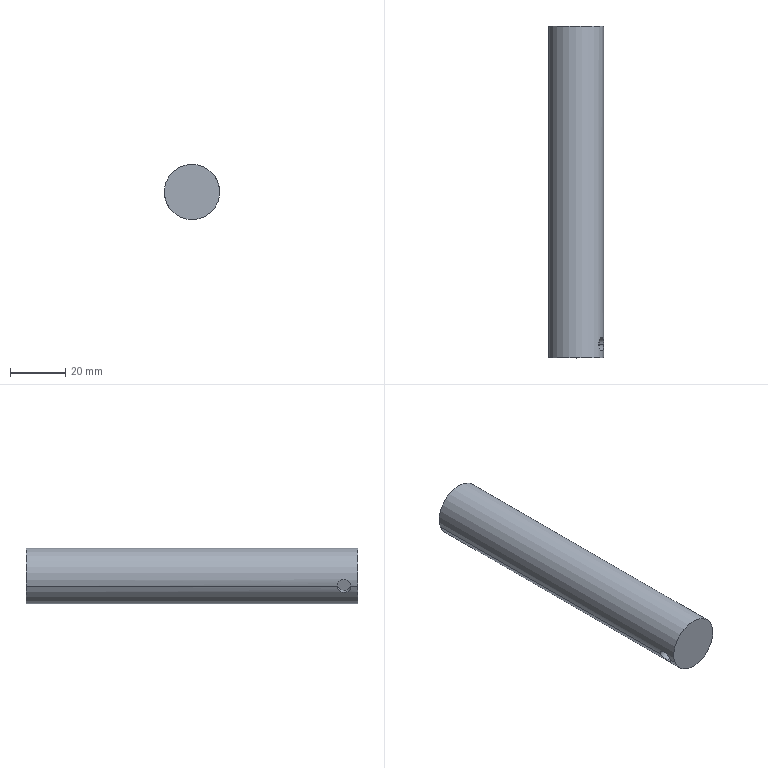Part | STEP file | Mirror 1-2 | 1 solid | 10 faces | box 20 x 120 x 20 mm | volume 37624 mm3 | cylinder 6 | plane 4 | commonest cylinder face diameters 5 x4 20 x2
STEP:
#1=CARTESIAN_POINT('',(-1482.225,1631.264,2822.025));
#2=VERTEX_POINT('',#1);
#3=CARTESIAN_POINT('',(-1480.38,1631.264,2817.378));
#4=VERTEX_POINT('',#3);
#5=CARTESIAN_POINT('',(-1481.302,1631.264,2819.702));
#6=DIRECTION('',(-0.9295,0.,-0.3689));
#7=DIRECTION('',(0.3689,0.,-0.9295));
#8=AXIS2_PLACEMENT_3D('',#5,#6,#7);
#9=CIRCLE('',#8,2.5);
#10=EDGE_CURVE('',#2,#4,#9,.T.);
#11=ORIENTED_EDGE('',*,*,#10,.T.);
#12=CARTESIAN_POINT('',(-1478.816,1631.264,2817.999));
#13=VERTEX_POINT('',#12);
#14=CARTESIAN_POINT('',(-1480.38,1631.264,2817.378));
#15=DIRECTION('',(-0.9295,0.,-0.3689));
#16=VECTOR('',#15,1000.);
#17=LINE('',#14,#16);
#18=EDGE_CURVE('',#13,#4,#17,.T.);
#19=ORIENTED_EDGE('',*,*,#18,.F.);
#20=CARTESIAN_POINT('',(-1479.444,1633.764,2820.44));
#21=VERTEX_POINT('',#20);
#22=CARTESIAN_POINT('',(-1478.816,1631.264,2817.999));
#23=CARTESIAN_POINT('',(-1478.816,1631.43,2817.999));
#24=CARTESIAN_POINT('',(-1478.819,1631.593,2818.016));
#25=CARTESIAN_POINT('',(-1478.827,1631.913,2818.081));
#26=CARTESIAN_POINT('',(-1478.834,1632.072,2818.13));
#27=CARTESIAN_POINT('',(-1478.852,1632.375,2818.258));
#28=CARTESIAN_POINT('',(-1478.864,1632.518,2818.336));
#29=CARTESIAN_POINT('',(-1478.895,1632.789,2818.518));
#30=CARTESIAN_POINT('',(-1478.915,1632.917,2818.624));
#31=CARTESIAN_POINT('',(-1478.984,1633.261,2818.966));
#32=CARTESIAN_POINT('',(-1479.048,1633.447,2819.239));
#33=CARTESIAN_POINT('',(-1479.174,1633.635,2819.674));
#34=CARTESIAN_POINT('',(-1479.221,1633.683,2819.825));
#35=CARTESIAN_POINT('',(-1479.326,1633.748,2820.132));
#36=CARTESIAN_POINT('',(-1479.382,1633.764,2820.286));
#37=CARTESIAN_POINT('',(-1479.444,1633.764,2820.44));
#38=B_SPLINE_CURVE_WITH_KNOTS('',3,(#22,#23,#24,#25,#26,#27,#28,#29,#30,#31,#32,#33,#34,#35,#36,#37),.UNSPECIFIED.,.F.,.F.,(4,2,2,2,2,2,2,4),(0.,0.0004901,0.0009802,0.00147,0.00196,0.002941,0.003431,0.003921),.UNSPECIFIED.);
#39=EDGE_CURVE('',#13,#21,#38,.T.);
#40=ORIENTED_EDGE('',*,*,#39,.T.);
#41=CARTESIAN_POINT('',(-1480.661,1631.264,2822.646));
#42=VERTEX_POINT('',#41);
#43=CARTESIAN_POINT('',(-1479.444,1633.764,2820.44));
#44=CARTESIAN_POINT('',(-1479.505,1633.764,2820.594));
#45=CARTESIAN_POINT('',(-1479.569,1633.748,2820.744));
#46=CARTESIAN_POINT('',(-1479.701,1633.684,2821.035));
#47=CARTESIAN_POINT('',(-1479.771,1633.636,2821.179));
#48=CARTESIAN_POINT('',(-1479.909,1633.51,2821.449));
#49=CARTESIAN_POINT('',(-1479.978,1633.433,2821.576));
#50=CARTESIAN_POINT('',(-1480.114,1633.252,2821.814));
#51=CARTESIAN_POINT('',(-1480.18,1633.147,2821.925));
#52=CARTESIAN_POINT('',(-1480.365,1632.803,2822.222));
#53=CARTESIAN_POINT('',(-1480.472,1632.525,2822.38));
#54=CARTESIAN_POINT('',(-1480.583,1632.075,2822.538));
#55=CARTESIAN_POINT('',(-1480.612,1631.917,2822.578));
#56=CARTESIAN_POINT('',(-1480.651,1631.594,2822.633));
#57=CARTESIAN_POINT('',(-1480.661,1631.43,2822.646));
#58=CARTESIAN_POINT('',(-1480.661,1631.264,2822.646));
#59=B_SPLINE_CURVE_WITH_KNOTS('',3,(#43,#44,#45,#46,#47,#48,#49,#50,#51,#52,#53,#54,#55,#56,#57,#58),.UNSPECIFIED.,.F.,.F.,(4,2,2,2,2,2,2,4),(0.,0.0004901,0.0009803,0.00147,0.001961,0.002941,0.003431,0.003921),.UNSPECIFIED.);
#60=EDGE_CURVE('',#21,#42,#59,.T.);
#61=ORIENTED_EDGE('',*,*,#60,.T.);
#62=CARTESIAN_POINT('',(-1482.225,1631.264,2822.025));
#63=DIRECTION('',(-0.9295,0.,-0.3689));
#64=VECTOR('',#63,1000.);
#65=LINE('',#62,#64);
#66=EDGE_CURVE('',#42,#2,#65,.T.);
#67=ORIENTED_EDGE('',*,*,#66,.T.);
#68=EDGE_LOOP('',(#11,#19,#40,#61,#67));
#69=FACE_OUTER_BOUND('',#68,.T.);
#70=CARTESIAN_POINT('',(-1481.302,1631.264,2819.702));
#71=DIRECTION('',(0.9295,0.,0.3689));
#72=DIRECTION('',(0.3689,0.,-0.9295));
#73=AXIS2_PLACEMENT_3D('',#70,#71,#72);
#74=CYLINDRICAL_SURFACE('',#73,2.5);
#75=ADVANCED_FACE('',(#69),#74,.F.);
#76=CARTESIAN_POINT('',(-1497.096,1631.264,2816.123));
#77=VERTEX_POINT('',#76);
#78=CARTESIAN_POINT('',(-1495.252,1631.264,2811.476));
#79=VERTEX_POINT('',#78);
#80=CARTESIAN_POINT('',(-1496.174,1631.264,2813.8));
#81=DIRECTION('',(-0.9295,0.,-0.3689));
#82=DIRECTION('',(0.3689,0.,-0.9295));
#83=AXIS2_PLACEMENT_3D('',#80,#81,#82);
#84=CIRCLE('',#83,2.5);
#85=EDGE_CURVE('',#77,#79,#84,.T.);
#86=ORIENTED_EDGE('',*,*,#85,.F.);
#87=CARTESIAN_POINT('',(-1498.66,1631.264,2815.503));
#88=VERTEX_POINT('',#87);
#89=CARTESIAN_POINT('',(-1497.096,1631.264,2816.123));
#90=DIRECTION('',(-0.9295,0.,-0.3689));
#91=VECTOR('',#90,1000.);
#92=LINE('',#89,#91);
#93=EDGE_CURVE('',#77,#88,#92,.T.);
#94=ORIENTED_EDGE('',*,*,#93,.T.);
#95=CARTESIAN_POINT('',(-1498.033,1633.764,2813.062));
#96=VERTEX_POINT('',#95);
#97=CARTESIAN_POINT('',(-1498.033,1633.764,2813.062));
#98=CARTESIAN_POINT('',(-1498.094,1633.764,2813.216));
#99=CARTESIAN_POINT('',(-1498.15,1633.748,2813.369));
#100=CARTESIAN_POINT('',(-1498.254,1633.684,2813.672));
#101=CARTESIAN_POINT('',(-1498.302,1633.636,2813.824));
#102=CARTESIAN_POINT('',(-1498.386,1633.51,2814.116));
#103=CARTESIAN_POINT('',(-1498.423,1633.433,2814.256));
#104=CARTESIAN_POINT('',(-1498.488,1633.252,2814.522));
#105=CARTESIAN_POINT('',(-1498.515,1633.147,2814.648));
#106=CARTESIAN_POINT('',(-1498.585,1632.803,2814.991));
#107=CARTESIAN_POINT('',(-1498.615,1632.525,2815.179));
#108=CARTESIAN_POINT('',(-1498.643,1632.075,2815.37));
#109=CARTESIAN_POINT('',(-1498.649,1631.917,2815.42));
#110=CARTESIAN_POINT('',(-1498.658,1631.594,2815.486));
#111=CARTESIAN_POINT('',(-1498.66,1631.43,2815.503));
#112=CARTESIAN_POINT('',(-1498.66,1631.264,2815.503));
#113=B_SPLINE_CURVE_WITH_KNOTS('',3,(#97,#98,#99,#100,#101,#102,#103,#104,#105,#106,#107,#108,#109,#110,#111,#112),.UNSPECIFIED.,.F.,.F.,(4,2,2,2,2,2,2,4),(0.,0.0004901,0.0009803,0.00147,0.001961,0.002941,0.003431,0.003921),.UNSPECIFIED.);
#114=EDGE_CURVE('',#96,#88,#113,.T.);
#115=ORIENTED_EDGE('',*,*,#114,.F.);
#116=CARTESIAN_POINT('',(-1496.816,1631.264,2810.855));
#117=VERTEX_POINT('',#116);
#118=CARTESIAN_POINT('',(-1496.816,1631.264,2810.855));
#119=CARTESIAN_POINT('',(-1496.816,1631.43,2810.855));
#120=CARTESIAN_POINT('',(-1496.826,1631.593,2810.869));
#121=CARTESIAN_POINT('',(-1496.864,1631.913,2810.922));
#122=CARTESIAN_POINT('',(-1496.893,1632.072,2810.963));
#123=CARTESIAN_POINT('',(-1496.967,1632.375,2811.068));
#124=CARTESIAN_POINT('',(-1497.012,1632.518,2811.133));
#125=CARTESIAN_POINT('',(-1497.115,1632.789,2811.287));
#126=CARTESIAN_POINT('',(-1497.173,1632.917,2811.377));
#127=CARTESIAN_POINT('',(-1497.357,1633.261,2811.674));
#128=CARTESIAN_POINT('',(-1497.498,1633.447,2811.917));
#129=CARTESIAN_POINT('',(-1497.704,1633.635,2812.32));
#130=CARTESIAN_POINT('',(-1497.774,1633.683,2812.462));
#131=CARTESIAN_POINT('',(-1497.908,1633.748,2812.757));
#132=CARTESIAN_POINT('',(-1497.972,1633.764,2812.908));
#133=CARTESIAN_POINT('',(-1498.033,1633.764,2813.062));
#134=B_SPLINE_CURVE_WITH_KNOTS('',3,(#118,#119,#120,#121,#122,#123,#124,#125,#126,#127,#128,#129,#130,#131,#132,#133),.UNSPECIFIED.,.F.,.F.,(4,2,2,2,2,2,2,4),(0.,0.0004901,0.0009802,0.00147,0.00196,0.002941,0.003431,0.003921),.UNSPECIFIED.);
#135=EDGE_CURVE('',#117,#96,#134,.T.);
#136=ORIENTED_EDGE('',*,*,#135,.F.);
#137=CARTESIAN_POINT('',(-1495.252,1631.264,2811.476));
#138=DIRECTION('',(-0.9295,0.,-0.3689));
#139=VECTOR('',#138,1000.);
#140=LINE('',#137,#139);
#141=EDGE_CURVE('',#79,#117,#140,.T.);
#142=ORIENTED_EDGE('',*,*,#141,.F.);
#143=EDGE_LOOP('',(#86,#94,#115,#136,#142));
#144=FACE_OUTER_BOUND('',#143,.T.);
#145=CARTESIAN_POINT('',(-1496.174,1631.264,2813.8));
#146=DIRECTION('',(-0.9295,0.,-0.3689));
#147=DIRECTION('',(-0.3689,0.,0.9295));
#148=AXIS2_PLACEMENT_3D('',#145,#146,#147);
#149=CYLINDRICAL_SURFACE('',#148,2.5);
#150=ADVANCED_FACE('',(#144),#149,.F.);
#151=CARTESIAN_POINT('',(-1498.033,1626.264,2813.062));
#152=VERTEX_POINT('',#151);
#153=CARTESIAN_POINT('',(-1479.444,1626.264,2820.44));
#154=VERTEX_POINT('',#153);
#155=CARTESIAN_POINT('',(-1488.738,1626.264,2816.751));
#156=DIRECTION('',(0.,-1.,0.));
#157=DIRECTION('',(-0.9295,0.,-0.3689));
#158=AXIS2_PLACEMENT_3D('',#155,#156,#157);
#159=CIRCLE('',#158,10.);
#160=EDGE_CURVE('',#152,#154,#159,.T.);
#161=ORIENTED_EDGE('',*,*,#160,.F.);
#162=CARTESIAN_POINT('',(-1498.033,1628.764,2813.062));
#163=VERTEX_POINT('',#162);
#164=CARTESIAN_POINT('',(-1498.033,1626.264,2813.062));
#165=DIRECTION('',(0.,-1.,0.));
#166=VECTOR('',#165,1000.);
#167=LINE('',#164,#166);
#168=EDGE_CURVE('',#163,#152,#167,.T.);
#169=ORIENTED_EDGE('',*,*,#168,.F.);
#170=CARTESIAN_POINT('',(-1498.033,1628.764,2813.062));
#171=CARTESIAN_POINT('',(-1497.972,1628.764,2812.908));
#172=CARTESIAN_POINT('',(-1497.908,1628.781,2812.758));
#173=CARTESIAN_POINT('',(-1497.775,1628.844,2812.466));
#174=CARTESIAN_POINT('',(-1497.706,1628.893,2812.322));
#175=CARTESIAN_POINT('',(-1497.567,1629.018,2812.052));
#176=CARTESIAN_POINT('',(-1497.498,1629.095,2811.925));
#177=CARTESIAN_POINT('',(-1497.363,1629.276,2811.687));
#178=CARTESIAN_POINT('',(-1497.296,1629.381,2811.576));
#179=CARTESIAN_POINT('',(-1497.112,1629.726,2811.279));
#180=CARTESIAN_POINT('',(-1497.004,1630.003,2811.121));
#181=CARTESIAN_POINT('',(-1496.894,1630.454,2810.964));
#182=CARTESIAN_POINT('',(-1496.865,1630.611,2810.923));
#183=CARTESIAN_POINT('',(-1496.826,1630.935,2810.869));
#184=CARTESIAN_POINT('',(-1496.816,1631.099,2810.855));
#185=CARTESIAN_POINT('',(-1496.816,1631.264,2810.855));
#186=B_SPLINE_CURVE_WITH_KNOTS('',3,(#170,#171,#172,#173,#174,#175,#176,#177,#178,#179,#180,#181,#182,#183,#184,#185),.UNSPECIFIED.,.F.,.F.,(4,2,2,2,2,2,2,4),(0.,0.0004901,0.0009803,0.00147,0.001961,0.002941,0.003431,0.003921),.UNSPECIFIED.);
#187=EDGE_CURVE('',#163,#117,#186,.T.);
#188=ORIENTED_EDGE('',*,*,#187,.T.);
#189=ORIENTED_EDGE('',*,*,#135,.T.);
#190=CARTESIAN_POINT('',(-1498.033,1746.264,2813.062));
#191=VERTEX_POINT('',#190);
#192=CARTESIAN_POINT('',(-1498.033,1626.264,2813.062));
#193=DIRECTION('',(0.,1.,0.));
#194=VECTOR('',#193,1000.);
#195=LINE('',#192,#194);
#196=EDGE_CURVE('',#96,#191,#195,.T.);
#197=ORIENTED_EDGE('',*,*,#196,.T.);
#198=CARTESIAN_POINT('',(-1479.444,1746.264,2820.44));
#199=VERTEX_POINT('',#198);
#200=CARTESIAN_POINT('',(-1488.738,1746.264,2816.751));
#201=DIRECTION('',(0.,-1.,0.));
#202=DIRECTION('',(-0.9295,0.,-0.3689));
#203=AXIS2_PLACEMENT_3D('',#200,#201,#202);
#204=CIRCLE('',#203,10.);
#205=EDGE_CURVE('',#191,#199,#204,.T.);
#206=ORIENTED_EDGE('',*,*,#205,.T.);
#207=CARTESIAN_POINT('',(-1479.444,1626.264,2820.44));
#208=DIRECTION('',(0.,-1.,0.));
#209=VECTOR('',#208,1000.);
#210=LINE('',#207,#209);
#211=EDGE_CURVE('',#199,#21,#210,.T.);
#212=ORIENTED_EDGE('',*,*,#211,.T.);
#213=ORIENTED_EDGE('',*,*,#39,.F.);
#214=CARTESIAN_POINT('',(-1479.444,1628.764,2820.44));
#215=VERTEX_POINT('',#214);
#216=CARTESIAN_POINT('',(-1479.444,1628.764,2820.44));
#217=CARTESIAN_POINT('',(-1479.382,1628.764,2820.286));
#218=CARTESIAN_POINT('',(-1479.326,1628.781,2820.133));
#219=CARTESIAN_POINT('',(-1479.223,1628.844,2819.829));
#220=CARTESIAN_POINT('',(-1479.175,1628.893,2819.677));
#221=CARTESIAN_POINT('',(-1479.09,1629.018,2819.385));
#222=CARTESIAN_POINT('',(-1479.054,1629.095,2819.246));
#223=CARTESIAN_POINT('',(-1478.989,1629.276,2818.98));
#224=CARTESIAN_POINT('',(-1478.961,1629.381,2818.853));
#225=CARTESIAN_POINT('',(-1478.892,1629.726,2818.51));
#226=CARTESIAN_POINT('',(-1478.862,1630.003,2818.322));
#227=CARTESIAN_POINT('',(-1478.834,1630.454,2818.131));
#228=CARTESIAN_POINT('',(-1478.827,1630.611,2818.082));
#229=CARTESIAN_POINT('',(-1478.819,1630.935,2818.016));
#230=CARTESIAN_POINT('',(-1478.816,1631.099,2817.999));
#231=CARTESIAN_POINT('',(-1478.816,1631.264,2817.999));
#232=B_SPLINE_CURVE_WITH_KNOTS('',3,(#216,#217,#218,#219,#220,#221,#222,#223,#224,#225,#226,#227,#228,#229,#230,#231),.UNSPECIFIED.,.F.,.F.,(4,2,2,2,2,2,2,4),(0.,0.0004901,0.0009803,0.00147,0.001961,0.002941,0.003431,0.003921),.UNSPECIFIED.);
#233=EDGE_CURVE('',#215,#13,#232,.T.);
#234=ORIENTED_EDGE('',*,*,#233,.F.);
#235=CARTESIAN_POINT('',(-1479.444,1626.264,2820.44));
#236=DIRECTION('',(0.,1.,0.));
#237=VECTOR('',#236,1000.);
#238=LINE('',#235,#237);
#239=EDGE_CURVE('',#154,#215,#238,.T.);
#240=ORIENTED_EDGE('',*,*,#239,.F.);
#241=EDGE_LOOP('',(#161,#169,#188,#189,#197,#206,#212,#213,#234,#240));
#242=FACE_OUTER_BOUND('',#241,.T.);
#243=CARTESIAN_POINT('',(-1488.738,1626.264,2816.751));
#244=DIRECTION('',(0.,1.,0.));
#245=DIRECTION('',(-0.9295,0.,-0.3689));
#246=AXIS2_PLACEMENT_3D('',#243,#244,#245);
#247=CYLINDRICAL_SURFACE('',#246,10.);
#248=ADVANCED_FACE('',(#242),#247,.T.);
#249=ORIENTED_EDGE('',*,*,#168,.T.);
#250=CARTESIAN_POINT('',(-1488.738,1626.264,2816.751));
#251=DIRECTION('',(0.,-1.,0.));
#252=DIRECTION('',(-0.9295,0.,-0.3689));
#253=AXIS2_PLACEMENT_3D('',#250,#251,#252);
#254=CIRCLE('',#253,10.);
#255=EDGE_CURVE('',#154,#152,#254,.T.);
#256=ORIENTED_EDGE('',*,*,#255,.F.);
#257=ORIENTED_EDGE('',*,*,#239,.T.);
#258=CARTESIAN_POINT('',(-1480.661,1631.264,2822.646));
#259=CARTESIAN_POINT('',(-1480.661,1631.099,2822.646));
#260=CARTESIAN_POINT('',(-1480.651,1630.936,2822.633));
#261=CARTESIAN_POINT('',(-1480.612,1630.615,2822.579));
#262=CARTESIAN_POINT('',(-1480.583,1630.456,2822.539));
#263=CARTESIAN_POINT('',(-1480.509,1630.154,2822.433));
#264=CARTESIAN_POINT('',(-1480.465,1630.011,2822.368));
#265=CARTESIAN_POINT('',(-1480.362,1629.74,2822.214));
#266=CARTESIAN_POINT('',(-1480.304,1629.612,2822.124));
#267=CARTESIAN_POINT('',(-1480.119,1629.268,2821.827));
#268=CARTESIAN_POINT('',(-1479.979,1629.081,2821.584));
#269=CARTESIAN_POINT('',(-1479.772,1628.894,2821.182));
#270=CARTESIAN_POINT('',(-1479.703,1628.845,2821.039));
#271=CARTESIAN_POINT('',(-1479.569,1628.781,2820.744));
#272=CARTESIAN_POINT('',(-1479.505,1628.764,2820.594));
#273=CARTESIAN_POINT('',(-1479.444,1628.764,2820.44));
#274=B_SPLINE_CURVE_WITH_KNOTS('',3,(#258,#259,#260,#261,#262,#263,#264,#265,#266,#267,#268,#269,#270,#271,#272,#273),.UNSPECIFIED.,.F.,.F.,(4,2,2,2,2,2,2,4),(0.,0.0004901,0.0009802,0.00147,0.00196,0.002941,0.003431,0.003921),.UNSPECIFIED.);
#275=EDGE_CURVE('',#42,#215,#274,.T.);
#276=ORIENTED_EDGE('',*,*,#275,.F.);
#277=ORIENTED_EDGE('',*,*,#60,.F.);
#278=ORIENTED_EDGE('',*,*,#211,.F.);
#279=CARTESIAN_POINT('',(-1488.738,1746.264,2816.751));
#280=DIRECTION('',(0.,-1.,0.));
#281=DIRECTION('',(-0.9295,0.,-0.3689));
#282=AXIS2_PLACEMENT_3D('',#279,#280,#281);
#283=CIRCLE('',#282,10.);
#284=EDGE_CURVE('',#199,#191,#283,.T.);
#285=ORIENTED_EDGE('',*,*,#284,.T.);
#286=ORIENTED_EDGE('',*,*,#196,.F.);
#287=ORIENTED_EDGE('',*,*,#114,.T.);
#288=CARTESIAN_POINT('',(-1498.66,1631.264,2815.503));
#289=CARTESIAN_POINT('',(-1498.66,1631.099,2815.503));
#290=CARTESIAN_POINT('',(-1498.658,1630.936,2815.486));
#291=CARTESIAN_POINT('',(-1498.649,1630.615,2815.421));
#292=CARTESIAN_POINT('',(-1498.643,1630.456,2815.371));
#293=CARTESIAN_POINT('',(-1498.624,1630.154,2815.244));
#294=CARTESIAN_POINT('',(-1498.612,1630.011,2815.166));
#295=CARTESIAN_POINT('',(-1498.581,1629.74,2814.983));
#296=CARTESIAN_POINT('',(-1498.562,1629.612,2814.878));
#297=CARTESIAN_POINT('',(-1498.493,1629.268,2814.535));
#298=CARTESIAN_POINT('',(-1498.428,1629.081,2814.262));
#299=CARTESIAN_POINT('',(-1498.303,1628.894,2813.827));
#300=CARTESIAN_POINT('',(-1498.255,1628.845,2813.676));
#301=CARTESIAN_POINT('',(-1498.151,1628.781,2813.37));
#302=CARTESIAN_POINT('',(-1498.094,1628.764,2813.216));
#303=CARTESIAN_POINT('',(-1498.033,1628.764,2813.062));
#304=B_SPLINE_CURVE_WITH_KNOTS('',3,(#288,#289,#290,#291,#292,#293,#294,#295,#296,#297,#298,#299,#300,#301,#302,#303),.UNSPECIFIED.,.F.,.F.,(4,2,2,2,2,2,2,4),(0.,0.0004901,0.0009802,0.00147,0.00196,0.002941,0.003431,0.003921),.UNSPECIFIED.);
#305=EDGE_CURVE('',#88,#163,#304,.T.);
#306=ORIENTED_EDGE('',*,*,#305,.T.);
#307=EDGE_LOOP('',(#249,#256,#257,#276,#277,#278,#285,#286,#287,#306));
#308=FACE_OUTER_BOUND('',#307,.T.);
#309=CARTESIAN_POINT('',(-1488.738,1626.264,2816.751));
#310=DIRECTION('',(0.,1.,0.));
#311=DIRECTION('',(-0.9295,0.,-0.3689));
#312=AXIS2_PLACEMENT_3D('',#309,#310,#311);
#313=CYLINDRICAL_SURFACE('',#312,10.);
#314=ADVANCED_FACE('',(#308),#313,.T.);
#315=ORIENTED_EDGE('',*,*,#255,.T.);
#316=ORIENTED_EDGE('',*,*,#160,.T.);
#317=EDGE_LOOP('',(#315,#316));
#318=FACE_OUTER_BOUND('',#317,.T.);
#319=CARTESIAN_POINT('',(-1488.738,1626.264,2816.751));
#320=DIRECTION('',(0.,-1.,0.));
#321=DIRECTION('',(0.9295,0.,0.3689));
#322=AXIS2_PLACEMENT_3D('',#319,#320,#321);
#323=PLANE('',#322);
#324=ADVANCED_FACE('',(#318),#323,.T.);
#325=ORIENTED_EDGE('',*,*,#284,.F.);
#326=ORIENTED_EDGE('',*,*,#205,.F.);
#327=EDGE_LOOP('',(#325,#326));
#328=FACE_OUTER_BOUND('',#327,.T.);
#329=CARTESIAN_POINT('',(-1488.738,1746.264,2816.751));
#330=DIRECTION('',(0.,-1.,0.));
#331=DIRECTION('',(0.9295,0.,0.3689));
#332=AXIS2_PLACEMENT_3D('',#329,#330,#331);
#333=PLANE('',#332);
#334=ADVANCED_FACE('',(#328),#333,.F.);
#335=ORIENTED_EDGE('',*,*,#93,.F.);
#336=CARTESIAN_POINT('',(-1496.174,1631.264,2813.8));
#337=DIRECTION('',(-0.9295,0.,-0.3689));
#338=DIRECTION('',(0.3689,0.,-0.9295));
#339=AXIS2_PLACEMENT_3D('',#336,#337,#338);
#340=CIRCLE('',#339,2.5);
#341=EDGE_CURVE('',#79,#77,#340,.T.);
#342=ORIENTED_EDGE('',*,*,#341,.F.);
#343=ORIENTED_EDGE('',*,*,#141,.T.);
#344=ORIENTED_EDGE('',*,*,#187,.F.);
#345=ORIENTED_EDGE('',*,*,#305,.F.);
#346=EDGE_LOOP('',(#335,#342,#343,#344,#345));
#347=FACE_OUTER_BOUND('',#346,.T.);
#348=CARTESIAN_POINT('',(-1496.174,1631.264,2813.8));
#349=DIRECTION('',(-0.9295,0.,-0.3689));
#350=DIRECTION('',(-0.3689,0.,0.9295));
#351=AXIS2_PLACEMENT_3D('',#348,#349,#350);
#352=CYLINDRICAL_SURFACE('',#351,2.5);
#353=ADVANCED_FACE('',(#347),#352,.F.);
#354=ORIENTED_EDGE('',*,*,#341,.T.);
#355=ORIENTED_EDGE('',*,*,#85,.T.);
#356=EDGE_LOOP('',(#354,#355));
#357=FACE_OUTER_BOUND('',#356,.T.);
#358=CARTESIAN_POINT('',(-1496.174,1631.264,2813.8));
#359=DIRECTION('',(-0.9295,0.,-0.3689));
#360=DIRECTION('',(-0.3689,0.,0.9295));
#361=AXIS2_PLACEMENT_3D('',#358,#359,#360);
#362=PLANE('',#361);
#363=ADVANCED_FACE('',(#357),#362,.T.);
#364=ORIENTED_EDGE('',*,*,#18,.T.);
#365=CARTESIAN_POINT('',(-1481.302,1631.264,2819.702));
#366=DIRECTION('',(-0.9295,0.,-0.3689));
#367=DIRECTION('',(0.3689,0.,-0.9295));
#368=AXIS2_PLACEMENT_3D('',#365,#366,#367);
#369=CIRCLE('',#368,2.5);
#370=EDGE_CURVE('',#4,#2,#369,.T.);
#371=ORIENTED_EDGE('',*,*,#370,.T.);
#372=ORIENTED_EDGE('',*,*,#66,.F.);
#373=ORIENTED_EDGE('',*,*,#275,.T.);
#374=ORIENTED_EDGE('',*,*,#233,.T.);
#375=EDGE_LOOP('',(#364,#371,#372,#373,#374));
#376=FACE_OUTER_BOUND('',#375,.T.);
#377=CARTESIAN_POINT('',(-1481.302,1631.264,2819.702));
#378=DIRECTION('',(0.9295,0.,0.3689));
#379=DIRECTION('',(0.3689,0.,-0.9295));
#380=AXIS2_PLACEMENT_3D('',#377,#378,#379);
#381=CYLINDRICAL_SURFACE('',#380,2.5);
#382=ADVANCED_FACE('',(#376),#381,.F.);
#383=ORIENTED_EDGE('',*,*,#10,.F.);
#384=ORIENTED_EDGE('',*,*,#370,.F.);
#385=EDGE_LOOP('',(#383,#384));
#386=FACE_OUTER_BOUND('',#385,.T.);
#387=CARTESIAN_POINT('',(-1481.302,1631.264,2819.702));
#388=DIRECTION('',(0.9295,0.,0.3689));
#389=DIRECTION('',(-0.3689,0.,0.9295));
#390=AXIS2_PLACEMENT_3D('',#387,#388,#389);
#391=PLANE('',#390);
#392=ADVANCED_FACE('',(#386),#391,.T.);
#393=CLOSED_SHELL('',(#75,#150,#248,#314,#324,#334,#353,#363,#382,#392));
#394=MANIFOLD_SOLID_BREP('',#393);
#395=CARTESIAN_POINT('',(0.,0.,0.));
#396=DIRECTION('',(0.,0.,1.));
#397=DIRECTION('',(1.,0.,0.));
#398=AXIS2_PLACEMENT_3D('',#395,#396,#397);
#399=(LENGTH_UNIT()NAMED_UNIT(*)SI_UNIT(.MILLI.,.METRE.));
#400=UNCERTAINTY_MEASURE_WITH_UNIT(LENGTH_MEASURE(0.00001),#399,'','');
#401=(NAMED_UNIT(*)PLANE_ANGLE_UNIT()SI_UNIT($,.RADIAN.));
#402=(NAMED_UNIT(*)SI_UNIT($,.STERADIAN.)SOLID_ANGLE_UNIT());
#403=(GEOMETRIC_REPRESENTATION_CONTEXT(3)GLOBAL_UNCERTAINTY_ASSIGNED_CONTEXT((#400))GLOBAL_UNIT_ASSIGNED_CONTEXT((#399,#401,#402))REPRESENTATION_CONTEXT('',''));
#404=ADVANCED_BREP_SHAPE_REPRESENTATION('',(#394,#398),#403);